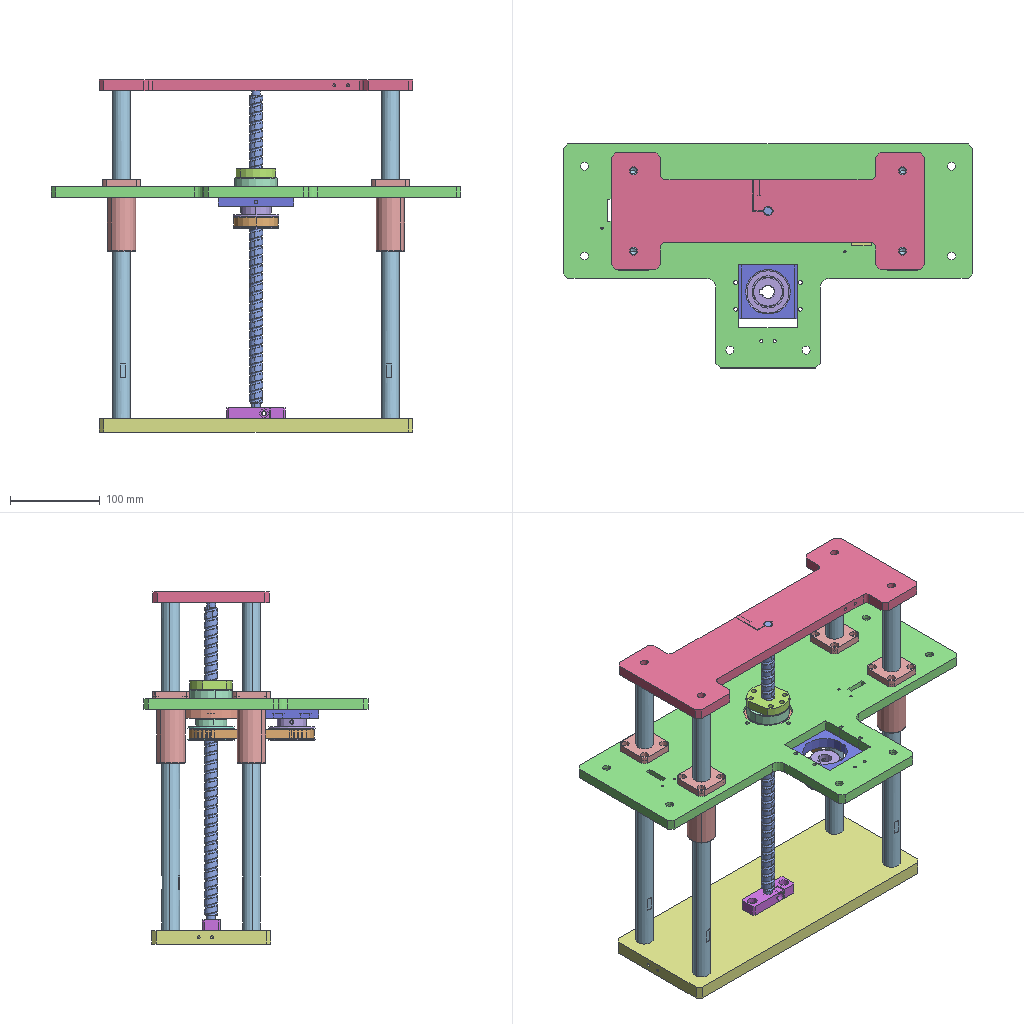Assembly | SolidWorks | 11 different items | 17 placed | box 456 x 250 x 393 mm
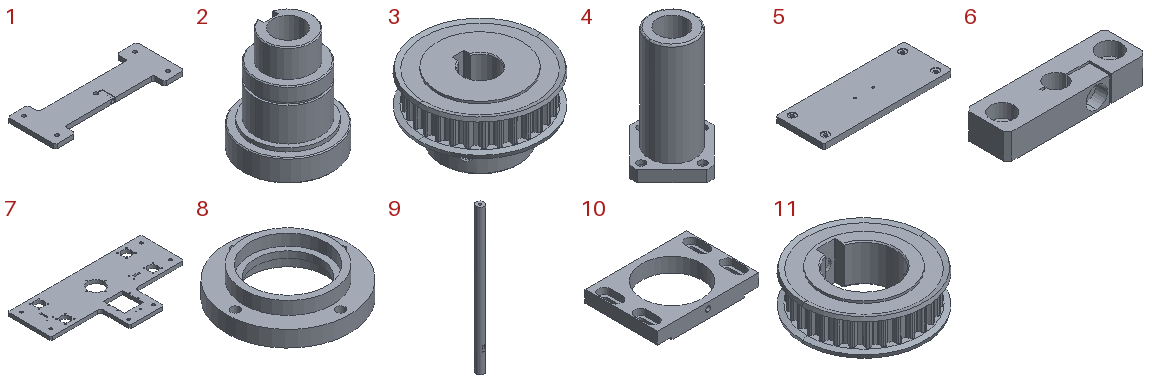Parts list (item | quantity | size | volume | features):
1 | x1 | 350 x 130 x 12 mm | 363525 mm3 | features HoleWzd 4, ICE 4, Chamfer 1, Extrusion 1, Fillet 1
2 | x1 | 48 x 48 x 56 mm | 29857 mm3 | features ICE 7, Chamfer 1, Extrusion 1, HoleWzd 1
3 | x1 | 52 x 52 x 28 mm | 31408 mm3 | features BaseBody 1
4 | x4 | 54 x 54 x 80 mm | 45045 mm3 | features BaseBody 1
5 | x1 | 350 x 133 x 15 mm | 687021 mm3 | features HoleWzd 3, Chamfer 1, Extrusion 1, ICE 1
6 | x1 | 65 x 20 x 12 mm | 12039 mm3 | features HoleWzd 3, ICE 2, Chamfer 1, Extrusion 1
7 | x1 | 456.5 x 250 x 12 mm | 820390 mm3 | features HoleWzd 6, ICE 5, Chamfer 1, Extrusion 1, Fillet 1
8 | x1 | 76 x 76 x 18 mm | 32922 mm3 | features ICE 4, Extrusion 1, HoleWzd 1
9 | x4 | 20 x 20 x 372 mm | 115321 mm3 | features HoleWzd 2, Extrusion 1, ICE 1
10 | x1 | 84 x 60 x 12 mm | 28663 mm3 | features HoleWzd 2, ICE 2, Extrusion 1
11 | x1 | 52 x 52 x 16 mm | 16805 mm3 | features BaseBody 1
Mates (type | each side: item.copy, entity, surface, feature):
Coincident | 1.1 face plane Cut-Extrude2 | 9.1 face plane Boss-Extrude1
Concentric | 1.1 face cylinder Cut-Extrude2 | 9.1 face cylinder Boss-Extrude1
Coincident | 5.1 face plane Boss-Extrude1 | 6.1 face plane Boss-Extrude1
Parallel | 7.1 face plane Boss-Extrude1 | 1.1 face plane Cut-Extrude1
Coincident | 7.1 face plane Boss-Extrude1 | 10.1 face plane Cut-Extrude3
Parallel | 7.1 face plane Boss-Extrude1 | 10.1 face plane Boss-Extrude1
Slot | 7.1 face cylinder M5 Tapped Hole3 | 10.1 face cylinder CBORE for M5 Hex Socket Head Cap Screw2
Coincident | 7.1 face plane Boss-Extrude1 | 8.1 face plane Boss-Extrude1
Concentric | 7.1 face cylinder M5 Tapped Hole2 | 8.1 face cylinder CBORE for M5 Hex Socket Head Cap Screw1 | 2 times
Concentric | 5.1 face cylinder M6 Tapped Hole1 | 6.1 face cylinder CBORE for M6 Hex Socket Head Cap Screw1 | 2 times
Concentric | 9.1 face cylinder Boss-Extrude1 | 4.1 face cylinder LMG13-d20
Concentric | 7.1 face cylinder M5 Tapped Hole1 | 4.1 face cylinder LMG13-d20 | 2 times
Coincident | 7.1 face plane Boss-Extrude1 | 4.1 face plane LMG13-d20
Coincident | 7.1 plane | assembly plane | 2 times
Coincident | 1.1 plane | assembly plane
Parallel | 11.1 face plane EBJ01-S5M100-30-A-N-d26 | 2.1 face plane Cut-Extrude3
Concentric | 11.1 face cylinder EBJ01-S5M100-30-A-N-d26 | 2.1 face cylinder Boss-Extrude4
Coincident | 11.1 face plane EBJ01-S5M100-30-A-N-d26 | 2.1 face plane Boss-Extrude3
Coincident | 11.1 face plane EBJ01-S5M100-30-A-N-d26 | 3.1 face plane EBJ01-S5M100-30-B-N-d14
Concentric | 9.1 face cylinder M8 Tapped Hole1 | 5.1 face cylinder CBORE for M8 Hex Socket Head Cap Screw1
Concentric | 5.1 face cylinder CBORE for M8 Hex Socket Head Cap Screw1 | 9.2 face cylinder M8 Tapped Hole1
LimitDistanceDim | 7.1 face plane Boss-Extrude1 | 1.1 face plane Boss-Extrude1